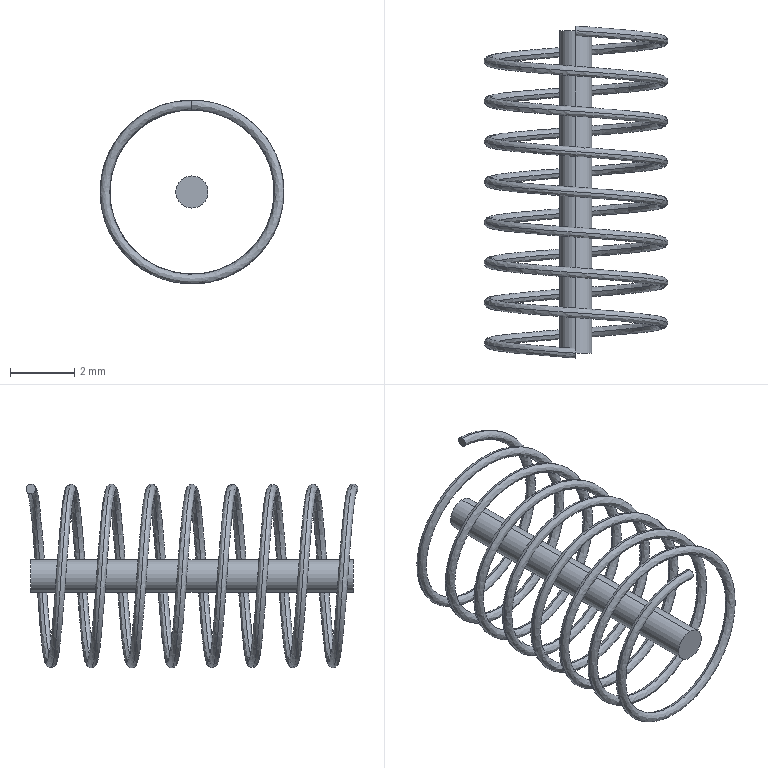Part | SolidWorks | features Helix 1, ICE 1, Sweep 1 | 2 solids | 8 faces | box 5.7 x 10.3 x 5.7 mm | volume 17.455 mm3 | plane 4 | spline 2 | cylinder 2 | commonest cylinder face diameters 1 x2